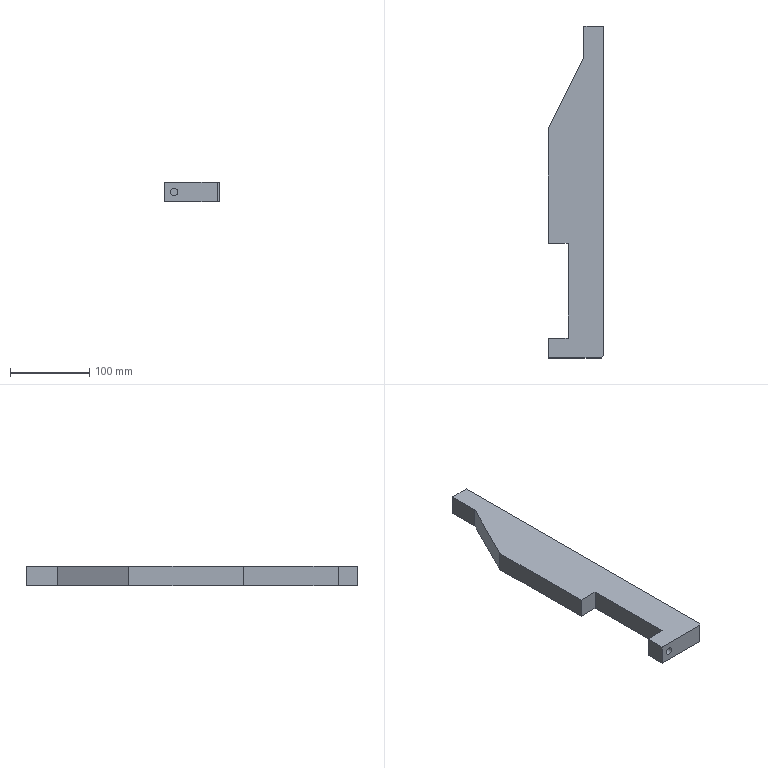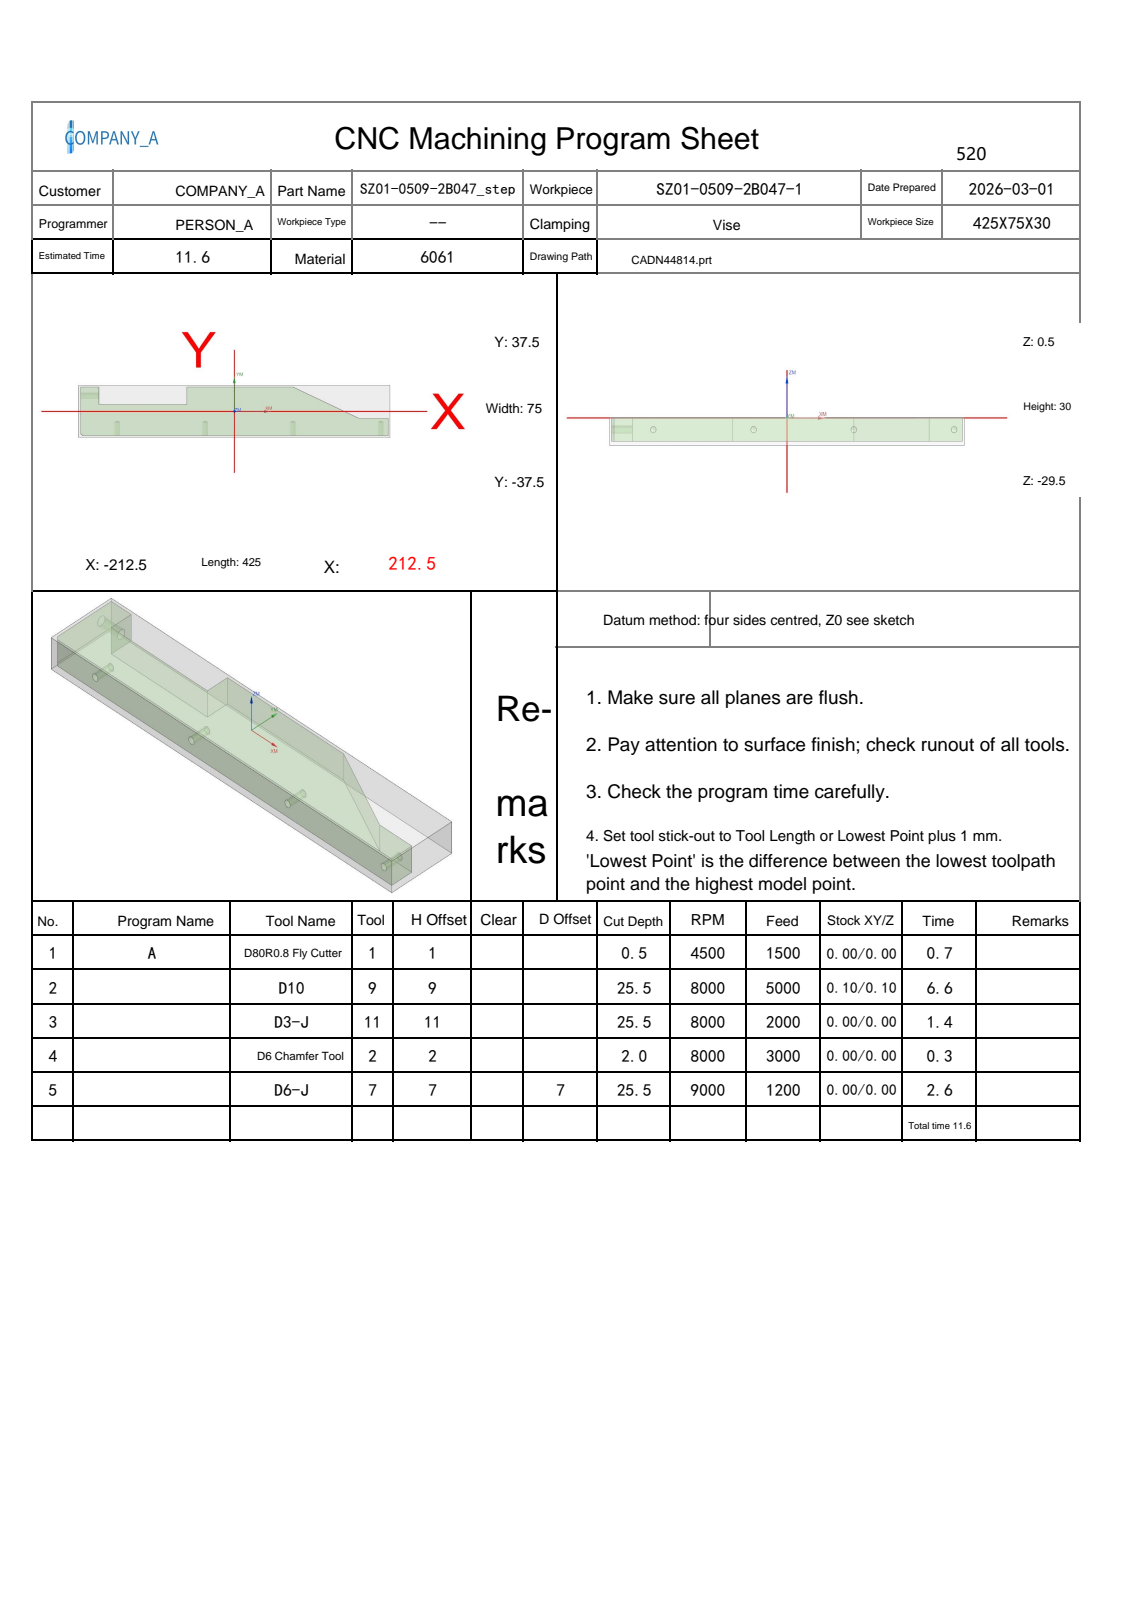NC program | NX | posted by the shop | part box 70 x 420 x 25 mm
Lines 3376 to 4374 of 10764:
N3 T11 M06
(D3-J  D=3. R=0. H=11 ce=0.00 di=0.00)
G00 G90 G54 X-183.199 Y15.275 M03 S8000
G43 H11 Z50.
M08
Z.05
G01 X-183.203 Y15.274 Z.004 F2000.
X-183.213 Y15.272 Z-.037
X-183.23 Y15.267 Z-.073
X-183.252 Y15.26 Z-.106
X-183.277 Y15.251 Z-.134
X-183.305 Y15.239 Z-.159
X-183.334 Y15.224 Z-.181
X-183.364 Y15.206 Z-.199
X-183.394 Y15.185 Z-.214
X-183.422 Y15.16 Z-.226
X-183.447 Y15.131 Z-.235
X-183.469 Y15.099 Z-.242
X-183.485 Y15.062 Z-.247
X-183.496 Y15.021 Z-.249
X-183.5 Y14.975 Z-.25
Y11.5
X-180.025
X-179.996 Y11.514 Z-.251
X-179.991 Y11.554 Z-.253
X-180.008 Y11.619 Z-.256
X-180.044 Y11.704 Z-.261
X-180.098 Y11.807 Z-.267
X-180.169 Y11.926 Z-.274
X-180.351 Y12.198 Z-.289
X-180.48 Y12.376 Z-.3
X-180.703 Y12.666 Z-.318
X-181.074 Y13.1 Z-.346
X-181.476 Y13.524 Z-.375
X-181.899 Y13.926 Z-.404
X-182.333 Y14.297 Z-.432
X-182.623 Y14.52 Z-.45
X-182.801 Y14.649 Z-.461
X-183.073 Y14.831 Z-.476
X-183.193 Y14.902 Z-.483
X-183.296 Y14.956 Z-.489
X-183.381 Y14.992 Z-.494
X-183.446 Y15.009 Z-.497
X-183.486 Y15.004 Z-.499
X-183.5 Y14.975 Z-.5
Y11.5
X-180.025
X-179.996 Y11.514 Z-.501
X-179.991 Y11.554 Z-.503
X-180.008 Y11.619 Z-.506
X-180.044 Y11.704 Z-.511
X-180.098 Y11.807 Z-.517
X-180.169 Y11.926 Z-.524
X-180.351 Y12.198 Z-.539
X-180.48 Y12.376 Z-.55
X-180.703 Y12.666 Z-.568
X-181.074 Y13.1 Z-.596
X-181.476 Y13.524 Z-.625
X-181.899 Y13.926 Z-.654
X-182.333 Y14.297 Z-.682
X-182.623 Y14.52 Z-.7
X-182.801 Y14.649 Z-.711
X-183.073 Y14.831 Z-.726
X-183.193 Y14.902 Z-.733
X-183.296 Y14.956 Z-.739
X-183.381 Y14.992 Z-.744
X-183.446 Y15.009 Z-.747
X-183.486 Y15.004 Z-.749
X-183.5 Y14.975 Z-.75
Y11.5
X-180.025
X-179.996 Y11.514 Z-.751
X-179.991 Y11.554 Z-.753
X-180.008 Y11.619 Z-.756
X-180.044 Y11.704 Z-.761
X-180.098 Y11.807 Z-.767
X-180.169 Y11.926 Z-.774
X-180.351 Y12.198 Z-.789
X-180.48 Y12.376 Z-.8
X-180.703 Y12.666 Z-.818
X-181.074 Y13.1 Z-.846
X-181.476 Y13.524 Z-.875
X-181.899 Y13.926 Z-.904
X-182.333 Y14.297 Z-.932
X-182.623 Y14.52 Z-.95
X-182.801 Y14.649 Z-.961
X-183.073 Y14.831 Z-.976
X-183.193 Y14.902 Z-.983
X-183.296 Y14.956 Z-.989
X-183.381 Y14.992 Z-.994
X-183.446 Y15.009 Z-.997
X-183.486 Y15.004 Z-.999
X-183.5 Y14.975 Z-1.
Y11.5
X-180.025
X-179.996 Y11.514 Z-1.001
X-179.991 Y11.554 Z-1.003
X-180.008 Y11.619 Z-1.006
X-180.044 Y11.704 Z-1.011
X-180.098 Y11.807 Z-1.017
X-180.169 Y11.926 Z-1.024
X-180.351 Y12.198 Z-1.039
X-180.48 Y12.376 Z-1.05
X-180.703 Y12.666 Z-1.068
X-181.074 Y13.1 Z-1.096
X-181.476 Y13.524 Z-1.125
X-181.899 Y13.926 Z-1.154
X-182.333 Y14.297 Z-1.182
X-182.623 Y14.52 Z-1.2
X-182.801 Y14.649 Z-1.211
X-183.073 Y14.831 Z-1.226
X-183.193 Y14.902 Z-1.233
X-183.296 Y14.956 Z-1.239
X-183.381 Y14.992 Z-1.244
X-183.446 Y15.009 Z-1.247
X-183.486 Y15.004 Z-1.249
X-183.5 Y14.975 Z-1.25
Y11.5
X-180.025
X-179.996 Y11.514 Z-1.251
X-179.991 Y11.554 Z-1.253
X-180.008 Y11.619 Z-1.256
X-180.044 Y11.704 Z-1.261
X-180.098 Y11.807 Z-1.267
X-180.169 Y11.926 Z-1.274
X-180.351 Y12.198 Z-1.289
X-180.48 Y12.376 Z-1.3
X-180.703 Y12.666 Z-1.318
X-181.074 Y13.1 Z-1.346
X-181.476 Y13.524 Z-1.375
X-181.899 Y13.926 Z-1.404
X-182.333 Y14.297 Z-1.432
X-182.623 Y14.52 Z-1.45
X-182.801 Y14.649 Z-1.461
X-183.073 Y14.831 Z-1.476
X-183.193 Y14.902 Z-1.483
X-183.296 Y14.956 Z-1.489
X-183.381 Y14.992 Z-1.494
X-183.446 Y15.009 Z-1.497
X-183.486 Y15.004 Z-1.499
X-183.5 Y14.975 Z-1.5
Y11.5
X-180.025
X-179.996 Y11.514 Z-1.501
X-179.991 Y11.554 Z-1.503
X-180.008 Y11.619 Z-1.506
X-180.044 Y11.704 Z-1.511
X-180.098 Y11.807 Z-1.517
X-180.169 Y11.926 Z-1.524
X-180.351 Y12.198 Z-1.539
X-180.48 Y12.376 Z-1.55
X-180.703 Y12.666 Z-1.568
X-181.074 Y13.1 Z-1.596
X-181.476 Y13.524 Z-1.625
X-181.899 Y13.926 Z-1.654
X-182.333 Y14.297 Z-1.682
X-182.623 Y14.52 Z-1.7
X-182.801 Y14.649 Z-1.711
X-183.073 Y14.831 Z-1.726
X-183.193 Y14.902 Z-1.733
X-183.296 Y14.956 Z-1.739
X-183.381 Y14.992 Z-1.744
X-183.446 Y15.009 Z-1.747
X-183.486 Y15.004 Z-1.749
X-183.5 Y14.975 Z-1.75
Y11.5
X-180.025
X-179.996 Y11.514 Z-1.751
X-179.991 Y11.554 Z-1.753
X-180.008 Y11.619 Z-1.756
X-180.044 Y11.704 Z-1.761
X-180.098 Y11.807 Z-1.767
X-180.169 Y11.926 Z-1.774
X-180.351 Y12.198 Z-1.789
X-180.48 Y12.376 Z-1.8
X-180.703 Y12.666 Z-1.818
X-181.074 Y13.1 Z-1.846
X-181.476 Y13.524 Z-1.875
X-181.899 Y13.926 Z-1.904
X-182.333 Y14.297 Z-1.932
X-182.623 Y14.52 Z-1.95
X-182.801 Y14.649 Z-1.961
X-183.073 Y14.831 Z-1.976
X-183.193 Y14.902 Z-1.983
X-183.296 Y14.956 Z-1.989
X-183.381 Y14.992 Z-1.994
X-183.446 Y15.009 Z-1.997
X-183.486 Y15.004 Z-1.999
X-183.5 Y14.975 Z-2.
Y11.5
X-180.025
X-179.996 Y11.514 Z-2.001
X-179.991 Y11.554 Z-2.003
X-180.008 Y11.619 Z-2.006
X-180.044 Y11.704 Z-2.011
X-180.098 Y11.807 Z-2.017
X-180.169 Y11.926 Z-2.024
X-180.351 Y12.198 Z-2.039
X-180.48 Y12.376 Z-2.05
X-180.703 Y12.666 Z-2.068
X-181.074 Y13.1 Z-2.096
X-181.476 Y13.524 Z-2.125
X-181.899 Y13.926 Z-2.154
X-182.333 Y14.297 Z-2.182
X-182.623 Y14.52 Z-2.2
X-182.801 Y14.649 Z-2.211
X-183.073 Y14.831 Z-2.226
X-183.193 Y14.902 Z-2.233
X-183.296 Y14.956 Z-2.239
X-183.381 Y14.992 Z-2.244
X-183.446 Y15.009 Z-2.247
X-183.486 Y15.004 Z-2.249
X-183.5 Y14.975 Z-2.25
Y11.5
X-180.025
X-179.996 Y11.514 Z-2.251
X-179.991 Y11.554 Z-2.253
X-180.008 Y11.619 Z-2.256
X-180.044 Y11.704 Z-2.261
X-180.098 Y11.807 Z-2.267
X-180.169 Y11.926 Z-2.274
X-180.351 Y12.198 Z-2.289
X-180.48 Y12.376 Z-2.3
X-180.703 Y12.666 Z-2.318
X-181.074 Y13.1 Z-2.346
X-181.476 Y13.524 Z-2.375
X-181.899 Y13.926 Z-2.404
X-182.333 Y14.297 Z-2.432
X-182.623 Y14.52 Z-2.45
X-182.801 Y14.649 Z-2.461
X-183.073 Y14.831 Z-2.476
X-183.193 Y14.902 Z-2.483
X-183.296 Y14.956 Z-2.489
X-183.381 Y14.992 Z-2.494
X-183.446 Y15.009 Z-2.497
X-183.486 Y15.004 Z-2.499
X-183.5 Y14.975 Z-2.5
Y11.5
X-180.025
X-179.996 Y11.514 Z-2.501
X-179.991 Y11.554 Z-2.503
X-180.008 Y11.619 Z-2.506
X-180.044 Y11.704 Z-2.511
X-180.098 Y11.807 Z-2.517
X-180.169 Y11.926 Z-2.524
X-180.351 Y12.198 Z-2.539
X-180.48 Y12.376 Z-2.55
X-180.703 Y12.666 Z-2.568
X-181.074 Y13.1 Z-2.596
X-181.476 Y13.524 Z-2.625
X-181.899 Y13.926 Z-2.654
X-182.333 Y14.297 Z-2.682
X-182.623 Y14.52 Z-2.7
X-182.801 Y14.649 Z-2.711
X-183.073 Y14.831 Z-2.726
X-183.193 Y14.902 Z-2.733
X-183.296 Y14.956 Z-2.739
X-183.381 Y14.992 Z-2.744
X-183.446 Y15.009 Z-2.747
X-183.486 Y15.004 Z-2.749
X-183.5 Y14.975 Z-2.75
Y11.5
X-180.025
X-179.996 Y11.514 Z-2.751
X-179.991 Y11.554 Z-2.753
X-180.008 Y11.619 Z-2.756
X-180.044 Y11.704 Z-2.761
X-180.098 Y11.807 Z-2.767
X-180.169 Y11.926 Z-2.774
X-180.351 Y12.198 Z-2.789
X-180.48 Y12.376 Z-2.8
X-180.703 Y12.666 Z-2.818
X-181.074 Y13.1 Z-2.846
X-181.476 Y13.524 Z-2.875
X-181.899 Y13.926 Z-2.904
X-182.333 Y14.297 Z-2.932
X-182.623 Y14.52 Z-2.95
X-182.801 Y14.649 Z-2.961
X-183.073 Y14.831 Z-2.976
X-183.193 Y14.902 Z-2.983
X-183.296 Y14.956 Z-2.989
X-183.381 Y14.992 Z-2.994
X-183.446 Y15.009 Z-2.997
X-183.486 Y15.004 Z-2.999
X-183.5 Y14.975 Z-3.
Y11.5
X-180.025
X-179.996 Y11.514 Z-3.001
X-179.991 Y11.554 Z-3.003
X-180.008 Y11.619 Z-3.006
X-180.044 Y11.704 Z-3.011
X-180.098 Y11.807 Z-3.017
X-180.169 Y11.926 Z-3.024
X-180.351 Y12.198 Z-3.039
X-180.48 Y12.376 Z-3.05
X-180.703 Y12.666 Z-3.068
X-181.074 Y13.1 Z-3.096
X-181.476 Y13.524 Z-3.125
X-181.899 Y13.926 Z-3.154
X-182.333 Y14.297 Z-3.182
X-182.623 Y14.52 Z-3.2
X-182.801 Y14.649 Z-3.211
X-183.073 Y14.831 Z-3.226
X-183.193 Y14.902 Z-3.233
X-183.296 Y14.956 Z-3.239
X-183.381 Y14.992 Z-3.244
X-183.446 Y15.009 Z-3.247
X-183.486 Y15.004 Z-3.249
X-183.5 Y14.975 Z-3.25
Y11.5
X-180.025
X-179.996 Y11.514 Z-3.251
X-179.991 Y11.554 Z-3.253
X-180.008 Y11.619 Z-3.256
X-180.044 Y11.704 Z-3.261
X-180.098 Y11.807 Z-3.267
X-180.169 Y11.926 Z-3.274
X-180.351 Y12.198 Z-3.289
X-180.48 Y12.376 Z-3.3
X-180.703 Y12.666 Z-3.318
X-181.074 Y13.1 Z-3.346
X-181.476 Y13.524 Z-3.375
X-181.899 Y13.926 Z-3.404
X-182.333 Y14.297 Z-3.432
X-182.623 Y14.52 Z-3.45
X-182.801 Y14.649 Z-3.461
X-183.073 Y14.831 Z-3.476
X-183.193 Y14.902 Z-3.483
X-183.296 Y14.956 Z-3.489
X-183.381 Y14.992 Z-3.494
X-183.446 Y15.009 Z-3.497
X-183.486 Y15.004 Z-3.499
X-183.5 Y14.975 Z-3.5
Y11.5
X-180.025
X-179.996 Y11.514 Z-3.501
X-179.991 Y11.554 Z-3.503
X-180.008 Y11.619 Z-3.506
X-180.044 Y11.704 Z-3.511
X-180.098 Y11.807 Z-3.517
X-180.169 Y11.926 Z-3.524
X-180.351 Y12.198 Z-3.539
X-180.48 Y12.376 Z-3.55
X-180.703 Y12.666 Z-3.568
X-181.074 Y13.1 Z-3.596
X-181.476 Y13.524 Z-3.625
X-181.899 Y13.926 Z-3.654
X-182.333 Y14.297 Z-3.682
X-182.623 Y14.52 Z-3.7
X-182.801 Y14.649 Z-3.711
X-183.073 Y14.831 Z-3.726
X-183.193 Y14.902 Z-3.733
X-183.296 Y14.956 Z-3.739
X-183.381 Y14.992 Z-3.744
X-183.446 Y15.009 Z-3.747
X-183.486 Y15.004 Z-3.749
X-183.5 Y14.975 Z-3.75
Y11.5
X-180.025
X-179.996 Y11.514 Z-3.751
X-179.991 Y11.554 Z-3.753
X-180.008 Y11.619 Z-3.756
X-180.044 Y11.704 Z-3.761
X-180.098 Y11.807 Z-3.767
X-180.169 Y11.926 Z-3.774
X-180.351 Y12.198 Z-3.789
X-180.48 Y12.376 Z-3.8
X-180.703 Y12.666 Z-3.818
X-181.074 Y13.1 Z-3.846
X-181.476 Y13.524 Z-3.875
X-181.899 Y13.926 Z-3.904
X-182.333 Y14.297 Z-3.932
X-182.623 Y14.52 Z-3.95
X-182.801 Y14.649 Z-3.961
X-183.073 Y14.831 Z-3.976
X-183.193 Y14.902 Z-3.983
X-183.296 Y14.956 Z-3.989
X-183.381 Y14.992 Z-3.994
X-183.446 Y15.009 Z-3.997
X-183.486 Y15.004 Z-3.999
X-183.5 Y14.975 Z-4.
Y11.5
X-180.025
X-179.996 Y11.514 Z-4.001
X-179.991 Y11.554 Z-4.003
X-180.008 Y11.619 Z-4.006
X-180.044 Y11.704 Z-4.011
X-180.098 Y11.807 Z-4.017
X-180.169 Y11.926 Z-4.024
X-180.351 Y12.198 Z-4.039
X-180.48 Y12.376 Z-4.05
X-180.703 Y12.666 Z-4.068
X-181.074 Y13.1 Z-4.096
X-181.476 Y13.524 Z-4.125
X-181.899 Y13.926 Z-4.154
X-182.333 Y14.297 Z-4.182
X-182.623 Y14.52 Z-4.2
X-182.801 Y14.649 Z-4.211
X-183.073 Y14.831 Z-4.226
X-183.193 Y14.902 Z-4.233
X-183.296 Y14.956 Z-4.239
X-183.381 Y14.992 Z-4.244
X-183.446 Y15.009 Z-4.247
X-183.486 Y15.004 Z-4.249
X-183.5 Y14.975 Z-4.25
Y11.5
X-180.025
X-179.996 Y11.514 Z-4.251
X-179.991 Y11.554 Z-4.253
X-180.008 Y11.619 Z-4.256
X-180.044 Y11.704 Z-4.261
X-180.098 Y11.807 Z-4.267
X-180.169 Y11.926 Z-4.274
X-180.351 Y12.198 Z-4.289
X-180.48 Y12.376 Z-4.3
X-180.703 Y12.666 Z-4.318
X-181.074 Y13.1 Z-4.346
X-181.476 Y13.524 Z-4.375
X-181.899 Y13.926 Z-4.404
X-182.333 Y14.297 Z-4.432
X-182.623 Y14.52 Z-4.45
X-182.801 Y14.649 Z-4.461
X-183.073 Y14.831 Z-4.476
X-183.193 Y14.902 Z-4.483
X-183.296 Y14.956 Z-4.489
X-183.381 Y14.992 Z-4.494
X-183.446 Y15.009 Z-4.497
X-183.486 Y15.004 Z-4.499
X-183.5 Y14.975 Z-4.5
Y11.5
X-180.025
X-179.996 Y11.514 Z-4.501
X-179.991 Y11.554 Z-4.503
X-180.008 Y11.619 Z-4.506
X-180.044 Y11.704 Z-4.511
X-180.098 Y11.807 Z-4.517
X-180.169 Y11.926 Z-4.524
X-180.351 Y12.198 Z-4.539
X-180.48 Y12.376 Z-4.55
X-180.703 Y12.666 Z-4.568
X-181.074 Y13.1 Z-4.596
X-181.476 Y13.524 Z-4.625
X-181.899 Y13.926 Z-4.654
X-182.333 Y14.297 Z-4.682
X-182.623 Y14.52 Z-4.7
X-182.801 Y14.649 Z-4.711
X-183.073 Y14.831 Z-4.726
X-183.193 Y14.902 Z-4.733
X-183.296 Y14.956 Z-4.739
X-183.381 Y14.992 Z-4.744
X-183.446 Y15.009 Z-4.747
X-183.486 Y15.004 Z-4.749
X-183.5 Y14.975 Z-4.75
Y11.5
X-180.025
X-179.996 Y11.514 Z-4.751
X-179.991 Y11.554 Z-4.753
X-180.008 Y11.619 Z-4.756
X-180.044 Y11.704 Z-4.761
X-180.098 Y11.807 Z-4.767
X-180.169 Y11.926 Z-4.774
X-180.351 Y12.198 Z-4.789
X-180.48 Y12.376 Z-4.8
X-180.703 Y12.666 Z-4.818
X-181.074 Y13.1 Z-4.846
X-181.476 Y13.524 Z-4.875
X-181.899 Y13.926 Z-4.904
X-182.333 Y14.297 Z-4.932
X-182.623 Y14.52 Z-4.95
X-182.801 Y14.649 Z-4.961
X-183.073 Y14.831 Z-4.976
X-183.193 Y14.902 Z-4.983
X-183.296 Y14.956 Z-4.989
X-183.381 Y14.992 Z-4.994
X-183.446 Y15.009 Z-4.997
X-183.486 Y15.004 Z-4.999
X-183.5 Y14.975 Z-5.
Y11.5
X-180.025
X-179.996 Y11.514 Z-5.001
X-179.991 Y11.554 Z-5.003
X-180.008 Y11.619 Z-5.006
X-180.044 Y11.704 Z-5.011
X-180.098 Y11.807 Z-5.017
X-180.169 Y11.926 Z-5.024
X-180.351 Y12.198 Z-5.039
X-180.48 Y12.376 Z-5.05
X-180.703 Y12.666 Z-5.068
X-181.074 Y13.1 Z-5.096
X-181.476 Y13.524 Z-5.125
X-181.899 Y13.926 Z-5.154
X-182.333 Y14.297 Z-5.182
X-182.623 Y14.52 Z-5.2
X-182.801 Y14.649 Z-5.211
X-183.073 Y14.831 Z-5.226
X-183.193 Y14.902 Z-5.233
X-183.296 Y14.956 Z-5.239
X-183.381 Y14.992 Z-5.244
X-183.446 Y15.009 Z-5.247
X-183.486 Y15.004 Z-5.249
X-183.5 Y14.975 Z-5.25
Y11.5
X-180.025
X-179.996 Y11.514 Z-5.251
X-179.991 Y11.554 Z-5.253
X-180.008 Y11.619 Z-5.256
X-180.044 Y11.704 Z-5.261
X-180.098 Y11.807 Z-5.267
X-180.169 Y11.926 Z-5.274
X-180.351 Y12.198 Z-5.289
X-180.48 Y12.376 Z-5.3
X-180.703 Y12.666 Z-5.318
X-181.074 Y13.1 Z-5.346
X-181.476 Y13.524 Z-5.375
X-181.899 Y13.926 Z-5.404
X-182.333 Y14.297 Z-5.432
X-182.623 Y14.52 Z-5.45
X-182.801 Y14.649 Z-5.461
X-183.073 Y14.831 Z-5.476
X-183.193 Y14.902 Z-5.483
X-183.296 Y14.956 Z-5.489
X-183.381 Y14.992 Z-5.494
X-183.446 Y15.009 Z-5.497
X-183.486 Y15.004 Z-5.499
X-183.5 Y14.975 Z-5.5
Y11.5
X-180.025
X-179.996 Y11.514 Z-5.501
X-179.991 Y11.554 Z-5.503
X-180.008 Y11.619 Z-5.506
X-180.044 Y11.704 Z-5.511
X-180.098 Y11.807 Z-5.517
X-180.169 Y11.926 Z-5.524
X-180.351 Y12.198 Z-5.539
X-180.48 Y12.376 Z-5.55
X-180.703 Y12.666 Z-5.568
X-181.074 Y13.1 Z-5.596
X-181.476 Y13.524 Z-5.625
X-181.899 Y13.926 Z-5.654
X-182.333 Y14.297 Z-5.682
X-182.623 Y14.52 Z-5.7
X-182.801 Y14.649 Z-5.711
X-183.073 Y14.831 Z-5.726
X-183.193 Y14.902 Z-5.733
X-183.296 Y14.956 Z-5.739
X-183.381 Y14.992 Z-5.744
X-183.446 Y15.009 Z-5.747
X-183.486 Y15.004 Z-5.749
X-183.5 Y14.975 Z-5.75
Y11.5
X-180.025
X-179.996 Y11.514 Z-5.751
X-179.991 Y11.554 Z-5.753
X-180.008 Y11.619 Z-5.756
X-180.044 Y11.704 Z-5.761
X-180.098 Y11.807 Z-5.767
X-180.169 Y11.926 Z-5.774
X-180.351 Y12.198 Z-5.789
X-180.48 Y12.376 Z-5.8
X-180.703 Y12.666 Z-5.818
X-181.074 Y13.1 Z-5.846
X-181.476 Y13.524 Z-5.875
X-181.899 Y13.926 Z-5.904
X-182.333 Y14.297 Z-5.932
X-182.623 Y14.52 Z-5.95
X-182.801 Y14.649 Z-5.961
X-183.073 Y14.831 Z-5.976
X-183.193 Y14.902 Z-5.983
X-183.296 Y14.956 Z-5.989
X-183.381 Y14.992 Z-5.994
X-183.446 Y15.009 Z-5.997
X-183.486 Y15.004 Z-5.999
X-183.5 Y14.975 Z-6.
Y11.5
X-180.025
X-179.996 Y11.514 Z-6.001
X-179.991 Y11.554 Z-6.003
X-180.008 Y11.619 Z-6.006
X-180.044 Y11.704 Z-6.011
X-180.098 Y11.807 Z-6.017
X-180.169 Y11.926 Z-6.024
X-180.351 Y12.198 Z-6.039
X-180.48 Y12.376 Z-6.05
X-180.703 Y12.666 Z-6.068
X-181.074 Y13.1 Z-6.096
X-181.476 Y13.524 Z-6.125
X-181.899 Y13.926 Z-6.154
X-182.333 Y14.297 Z-6.182
X-182.623 Y14.52 Z-6.2
X-182.801 Y14.649 Z-6.211
X-183.073 Y14.831 Z-6.226
X-183.193 Y14.902 Z-6.233
X-183.296 Y14.956 Z-6.239
X-183.381 Y14.992 Z-6.244
X-183.446 Y15.009 Z-6.247
X-183.486 Y15.004 Z-6.249
X-183.5 Y14.975 Z-6.25
Y11.5
X-180.025
X-179.996 Y11.514 Z-6.251
X-179.991 Y11.554 Z-6.253
X-180.008 Y11.619 Z-6.256
X-180.044 Y11.704 Z-6.261
X-180.098 Y11.807 Z-6.267
X-180.169 Y11.926 Z-6.274
X-180.351 Y12.198 Z-6.289
X-180.48 Y12.376 Z-6.3
X-180.703 Y12.666 Z-6.318
X-181.074 Y13.1 Z-6.346
X-181.476 Y13.524 Z-6.375
X-181.899 Y13.926 Z-6.404
X-182.333 Y14.297 Z-6.432
X-182.623 Y14.52 Z-6.45
X-182.801 Y14.649 Z-6.461
X-183.073 Y14.831 Z-6.476
X-183.193 Y14.902 Z-6.483
X-183.296 Y14.956 Z-6.489
X-183.381 Y14.992 Z-6.494
X-183.446 Y15.009 Z-6.497
X-183.486 Y15.004 Z-6.499
X-183.5 Y14.975 Z-6.5
Y11.5
X-180.025
X-179.996 Y11.514 Z-6.501
X-179.991 Y11.554 Z-6.503
X-180.008 Y11.619 Z-6.506
X-180.044 Y11.704 Z-6.511
X-180.098 Y11.807 Z-6.517
X-180.169 Y11.926 Z-6.524
X-180.351 Y12.198 Z-6.539
X-180.48 Y12.376 Z-6.55
X-180.703 Y12.666 Z-6.568
X-181.074 Y13.1 Z-6.596
X-181.476 Y13.524 Z-6.625
X-181.899 Y13.926 Z-6.654
X-182.333 Y14.297 Z-6.682
X-182.623 Y14.52 Z-6.7
X-182.801 Y14.649 Z-6.711
X-183.073 Y14.831 Z-6.726
X-183.193 Y14.902 Z-6.733
X-183.296 Y14.956 Z-6.739
X-183.381 Y14.992 Z-6.744
X-183.446 Y15.009 Z-6.747
X-183.486 Y15.004 Z-6.749
X-183.5 Y14.975 Z-6.75
Y11.5
X-180.025
X-179.996 Y11.514 Z-6.751
X-179.991 Y11.554 Z-6.753
X-180.008 Y11.619 Z-6.756
X-180.044 Y11.704 Z-6.761
X-180.098 Y11.807 Z-6.767
X-180.169 Y11.926 Z-6.774
X-180.351 Y12.198 Z-6.789
X-180.48 Y12.376 Z-6.8
X-180.703 Y12.666 Z-6.818
X-181.074 Y13.1 Z-6.846
X-181.476 Y13.524 Z-6.875
X-181.899 Y13.926 Z-6.904
X-182.333 Y14.297 Z-6.932
X-182.623 Y14.52 Z-6.95
X-182.801 Y14.649 Z-6.961
X-183.073 Y14.831 Z-6.976
X-183.193 Y14.902 Z-6.983
X-183.296 Y14.956 Z-6.989
X-183.381 Y14.992 Z-6.994
X-183.446 Y15.009 Z-6.997
X-183.486 Y15.004 Z-6.999
X-183.5 Y14.975 Z-7.
Y11.5
X-180.025
X-179.996 Y11.514 Z-7.001
X-179.991 Y11.554 Z-7.003
X-180.008 Y11.619 Z-7.006
X-180.044 Y11.704 Z-7.011
X-180.098 Y11.807 Z-7.017
X-180.169 Y11.926 Z-7.024
X-180.351 Y12.198 Z-7.039
X-180.48 Y12.376 Z-7.05
X-180.703 Y12.666 Z-7.068
X-181.074 Y13.1 Z-7.096
X-181.476 Y13.524 Z-7.125
X-181.899 Y13.926 Z-7.154
X-182.333 Y14.297 Z-7.182
X-182.623 Y14.52 Z-7.2
X-182.801 Y14.649 Z-7.211
X-183.073 Y14.831 Z-7.226
X-183.193 Y14.902 Z-7.233
X-183.296 Y14.956 Z-7.239
X-183.381 Y14.992 Z-7.244
X-183.446 Y15.009 Z-7.247
X-183.486 Y15.004 Z-7.249
X-183.5 Y14.975 Z-7.25
Y11.5
X-180.025
X-179.996 Y11.514 Z-7.251
X-179.991 Y11.554 Z-7.253
X-180.008 Y11.619 Z-7.256
X-180.044 Y11.704 Z-7.261
X-180.098 Y11.807 Z-7.267
X-180.169 Y11.926 Z-7.274
X-180.351 Y12.198 Z-7.289
X-180.48 Y12.376 Z-7.3
X-180.703 Y12.666 Z-7.318
X-181.074 Y13.1 Z-7.346
X-181.476 Y13.524 Z-7.375
X-181.899 Y13.926 Z-7.404
X-182.333 Y14.297 Z-7.432
X-182.623 Y14.52 Z-7.45
X-182.801 Y14.649 Z-7.461
X-183.073 Y14.831 Z-7.476
X-183.193 Y14.902 Z-7.483
X-183.296 Y14.956 Z-7.489
X-183.381 Y14.992 Z-7.494
X-183.446 Y15.009 Z-7.497
X-183.486 Y15.004 Z-7.499
X-183.5 Y14.975 Z-7.5
Y11.5
X-180.025
X-179.996 Y11.514 Z-7.501
X-179.991 Y11.554 Z-7.503
X-180.008 Y11.619 Z-7.506
X-180.044 Y11.704 Z-7.511
X-180.098 Y11.807 Z-7.517
X-180.169 Y11.926 Z-7.524
X-180.351 Y12.198 Z-7.539
X-180.48 Y12.376 Z-7.55
X-180.703 Y12.666 Z-7.568
X-181.074 Y13.1 Z-7.596
X-181.476 Y13.524 Z-7.625
X-181.899 Y13.926 Z-7.654
X-182.333 Y14.297 Z-7.682
X-182.623 Y14.52 Z-7.7
X-182.801 Y14.649 Z-7.711
X-183.073 Y14.831 Z-7.726
X-183.193 Y14.902 Z-7.733
X-183.296 Y14.956 Z-7.739
X-183.381 Y14.992 Z-7.744
X-183.446 Y15.009 Z-7.747
X-183.486 Y15.004 Z-7.749
X-183.5 Y14.975 Z-7.75
Y11.5
X-180.025
X-179.996 Y11.514 Z-7.751
X-179.991 Y11.554 Z-7.753
X-180.008 Y11.619 Z-7.756
X-180.044 Y11.704 Z-7.761
X-180.098 Y11.807 Z-7.767
X-180.169 Y11.926 Z-7.774
X-180.351 Y12.198 Z-7.789
X-180.48 Y12.376 Z-7.8
X-180.703 Y12.666 Z-7.818
X-181.074 Y13.1 Z-7.846
X-181.476 Y13.524 Z-7.875
X-181.899 Y13.926 Z-7.904
X-182.333 Y14.297 Z-7.932
X-182.623 Y14.52 Z-7.95
X-182.801 Y14.649 Z-7.961
X-183.073 Y14.831 Z-7.976
X-183.193 Y14.902 Z-7.983
X-183.296 Y14.956 Z-7.989
X-183.381 Y14.992 Z-7.994
X-183.446 Y15.009 Z-7.997
X-183.486 Y15.004 Z-7.999
X-183.5 Y14.975 Z-8.
Y11.5
X-180.025
X-179.996 Y11.514 Z-8.001
X-179.991 Y11.554 Z-8.003
X-180.008 Y11.619 Z-8.006
X-180.044 Y11.704 Z-8.011
X-180.098 Y11.807 Z-8.017
X-180.169 Y11.926 Z-8.024
X-180.351 Y12.198 Z-8.039
X-180.48 Y12.376 Z-8.05
X-180.703 Y12.666 Z-8.068
X-181.074 Y13.1 Z-8.096
X-181.476 Y13.524 Z-8.125
X-181.899 Y13.926 Z-8.154
X-182.333 Y14.297 Z-8.182
X-182.623 Y14.52 Z-8.2
X-182.801 Y14.649 Z-8.211
X-183.073 Y14.831 Z-8.226
X-183.193 Y14.902 Z-8.233
X-183.296 Y14.956 Z-8.239
X-183.381 Y14.992 Z-8.244
X-183.446 Y15.009 Z-8.247
X-183.486 Y15.004 Z-8.249
X-183.5 Y14.975 Z-8.25
Y11.5
X-180.025
X-179.996 Y11.514 Z-8.251
X-179.991 Y11.554 Z-8.253
X-180.008 Y11.619 Z-8.256
X-180.044 Y11.704 Z-8.261
X-180.098 Y11.807 Z-8.267
X-180.169 Y11.926 Z-8.274
X-180.351 Y12.198 Z-8.289
X-180.48 Y12.376 Z-8.3
X-180.703 Y12.666 Z-8.318
X-181.074 Y13.1 Z-8.346
X-181.476 Y13.524 Z-8.375
X-181.899 Y13.926 Z-8.404
X-182.333 Y14.297 Z-8.432
X-182.623 Y14.52 Z-8.45
X-182.801 Y14.649 Z-8.461
X-183.073 Y14.831 Z-8.476
X-183.193 Y14.902 Z-8.483
X-183.296 Y14.956 Z-8.489
X-183.381 Y14.992 Z-8.494
X-183.446 Y15.009 Z-8.497
X-183.486 Y15.004 Z-8.499
X-183.5 Y14.975 Z-8.5
Y11.5
X-180.025
X-179.996 Y11.514 Z-8.501
X-179.991 Y11.554 Z-8.503
X-180.008 Y11.619 Z-8.506
X-180.044 Y11.704 Z-8.511
X-180.098 Y11.807 Z-8.517
X-180.169 Y11.926 Z-8.524
X-180.351 Y12.198 Z-8.539
X-180.48 Y12.376 Z-8.55
X-180.703 Y12.666 Z-8.568
X-181.074 Y13.1 Z-8.596
X-181.476 Y13.524 Z-8.625
X-181.899 Y13.926 Z-8.654
X-182.333 Y14.297 Z-8.682
X-182.623 Y14.52 Z-8.7
X-182.801 Y14.649 Z-8.711
X-183.073 Y14.831 Z-8.726
X-183.193 Y14.902 Z-8.733
X-183.296 Y14.956 Z-8.739
X-183.381 Y14.992 Z-8.744
X-183.446 Y15.009 Z-8.747
X-183.486 Y15.004 Z-8.749
X-183.5 Y14.975 Z-8.75
Y11.5
X-180.025
X-179.996 Y11.514 Z-8.751
X-179.991 Y11.554 Z-8.753
X-180.008 Y11.619 Z-8.756
X-180.044 Y11.704 Z-8.761
X-180.098 Y11.807 Z-8.767
X-180.169 Y11.926 Z-8.774
X-180.351 Y12.198 Z-8.789
X-180.48 Y12.376 Z-8.8
X-180.703 Y12.666 Z-8.818
X-181.074 Y13.1 Z-8.846
X-181.476 Y13.524 Z-8.875
X-181.899 Y13.926 Z-8.904
X-182.333 Y14.297 Z-8.932
X-182.623 Y14.52 Z-8.95
X-182.801 Y14.649 Z-8.961
X-183.073 Y14.831 Z-8.976
X-183.193 Y14.902 Z-8.983
X-183.296 Y14.956 Z-8.989
X-183.381 Y14.992 Z-8.994
X-183.446 Y15.009 Z-8.997
X-183.486 Y15.004 Z-8.999
X-183.5 Y14.975 Z-9.
Y11.5
X-180.025
X-179.996 Y11.514 Z-9.001
X-179.991 Y11.554 Z-9.003
X-180.008 Y11.619 Z-9.006
X-180.044 Y11.704 Z-9.011
X-180.098 Y11.807 Z-9.017
X-180.169 Y11.926 Z-9.024
X-180.351 Y12.198 Z-9.039
X-180.48 Y12.376 Z-9.05
X-180.703 Y12.666 Z-9.068
X-181.074 Y13.1 Z-9.096
X-181.476 Y13.524 Z-9.125
X-181.899 Y13.926 Z-9.154
X-182.333 Y14.297 Z-9.182
X-182.623 Y14.52 Z-9.2
X-182.801 Y14.649 Z-9.211
X-183.073 Y14.831 Z-9.226
X-183.193 Y14.902 Z-9.233
X-183.296 Y14.956 Z-9.239
X-183.381 Y14.992 Z-9.244
X-183.446 Y15.009 Z-9.247
X-183.486 Y15.004 Z-9.249
X-183.5 Y14.975 Z-9.25
Y11.5
X-180.025
X-179.996 Y11.514 Z-9.251
X-179.991 Y11.554 Z-9.253
X-180.008 Y11.619 Z-9.256
X-180.044 Y11.704 Z-9.261
X-180.098 Y11.807 Z-9.267
X-180.169 Y11.926 Z-9.274
X-180.351 Y12.198 Z-9.289
X-180.48 Y12.376 Z-9.3
X-180.703 Y12.666 Z-9.318
X-181.074 Y13.1 Z-9.346
X-181.476 Y13.524 Z-9.375
X-181.899 Y13.926 Z-9.404
X-182.333 Y14.297 Z-9.432
X-182.623 Y14.52 Z-9.45
X-182.801 Y14.649 Z-9.461
X-183.073 Y14.831 Z-9.476
X-183.193 Y14.902 Z-9.483
X-183.296 Y14.956 Z-9.489
X-183.381 Y14.992 Z-9.494
X-183.446 Y15.009 Z-9.497
X-183.486 Y15.004 Z-9.499
X-183.5 Y14.975 Z-9.5
Y11.5
X-180.025
X-179.996 Y11.514 Z-9.501
X-179.991 Y11.554 Z-9.503
X-180.008 Y11.619 Z-9.506
X-180.044 Y11.704 Z-9.511
X-180.098 Y11.807 Z-9.517
X-180.169 Y11.926 Z-9.524
X-180.351 Y12.198 Z-9.539
X-180.48 Y12.376 Z-9.55
X-180.703 Y12.666 Z-9.568
X-181.074 Y13.1 Z-9.596
X-181.476 Y13.524 Z-9.625
X-181.899 Y13.926 Z-9.654
X-182.333 Y14.297 Z-9.682
X-182.623 Y14.52 Z-9.7
X-182.801 Y14.649 Z-9.711
X-183.073 Y14.831 Z-9.726
X-183.193 Y14.902 Z-9.733
X-183.296 Y14.956 Z-9.739
X-183.381 Y14.992 Z-9.744
X-183.446 Y15.009 Z-9.747
X-183.486 Y15.004 Z-9.749
X-183.5 Y14.975 Z-9.75
Y11.5
X-180.025
X-179.996 Y11.514 Z-9.751
X-179.991 Y11.554 Z-9.753
X-180.008 Y11.619 Z-9.756
X-180.044 Y11.704 Z-9.761
X-180.098 Y11.807 Z-9.767
X-180.169 Y11.926 Z-9.774
X-180.351 Y12.198 Z-9.789
X-180.48 Y12.376 Z-9.8
X-180.703 Y12.666 Z-9.818
X-181.074 Y13.1 Z-9.846
X-181.476 Y13.524 Z-9.875
X-181.899 Y13.926 Z-9.904
X-182.333 Y14.297 Z-9.932
X-182.623 Y14.52 Z-9.95
X-182.801 Y14.649 Z-9.961
X-183.073 Y14.831 Z-9.976
X-183.193 Y14.902 Z-9.983
X-183.296 Y14.956 Z-9.989
X-183.381 Y14.992 Z-9.994
X-183.446 Y15.009 Z-9.997
X-183.486 Y15.004 Z-9.999
X-183.5 Y14.975 Z-10.
Y11.5
X-180.025
X-179.996 Y11.514 Z-10.001
X-179.991 Y11.554 Z-10.003
X-180.008 Y11.619 Z-10.006
X-180.044 Y11.704 Z-10.011
X-180.098 Y11.807 Z-10.017
X-180.169 Y11.926 Z-10.024
X-180.351 Y12.198 Z-10.039
X-180.48 Y12.376 Z-10.05
X-180.703 Y12.666 Z-10.068
X-181.074 Y13.1 Z-10.096
X-181.476 Y13.524 Z-10.125
X-181.899 Y13.926 Z-10.154
X-182.333 Y14.297 Z-10.182
X-182.623 Y14.52 Z-10.2
X-182.801 Y14.649 Z-10.211
X-183.073 Y14.831 Z-10.226
X-183.193 Y14.902 Z-10.233
X-183.296 Y14.956 Z-10.239
X-183.381 Y14.992 Z-10.244
X-183.446 Y15.009 Z-10.247
X-183.486 Y15.004 Z-10.249
X-183.5 Y14.975 Z-10.25
Y11.5
X-180.025
X-179.996 Y11.514 Z-10.251
X-179.991 Y11.554 Z-10.253
X-180.008 Y11.619 Z-10.256
X-180.044 Y11.704 Z-10.261
X-180.098 Y11.807 Z-10.267
X-180.169 Y11.926 Z-10.274
X-180.351 Y12.198 Z-10.289
X-180.48 Y12.376 Z-10.3
X-180.703 Y12.666 Z-10.318
X-181.074 Y13.1 Z-10.346
X-181.476 Y13.524 Z-10.375
X-181.899 Y13.926 Z-10.404
X-182.333 Y14.297 Z-10.432
X-182.623 Y14.52 Z-10.45
X-182.801 Y14.649 Z-10.461
X-183.073 Y14.831 Z-10.476